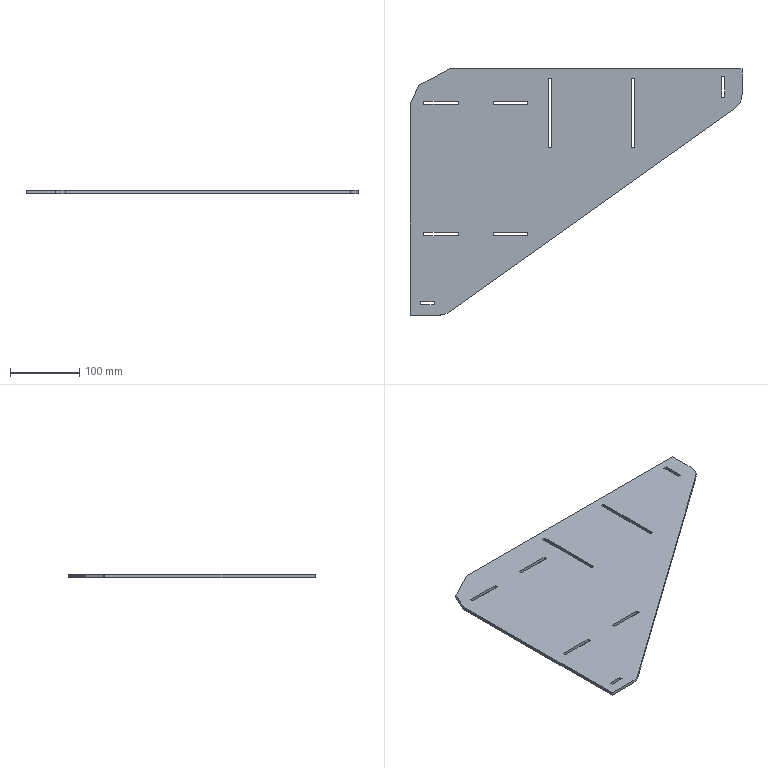Part | SolidWorks | features FlatPattern 1, SMBaseFlange 1, SheetMetal 1 | 1 solid | 44 faces | box 479.97 x 356 x 4.5 mm | volume 459091 mm3 | plane 42 | cylinder 2 | commonest cylinder face diameters 50 x2
STEP:
#1=CARTESIAN_POINT('',(28.5,449.2,0.));
#2=VERTEX_POINT('',#1);
#3=CARTESIAN_POINT('',(70.512,449.2,0.));
#4=VERTEX_POINT('',#3);
#5=CARTESIAN_POINT('',(28.5,449.2,0.));
#6=DIRECTION('',(1.,0.,0.));
#7=VECTOR('',#6,1000.);
#8=LINE('',#5,#7);
#9=EDGE_CURVE('',#2,#4,#8,.T.);
#10=ORIENTED_EDGE('',*,*,#9,.F.);
#11=CARTESIAN_POINT('',(28.5,449.2,-4.5));
#12=VERTEX_POINT('',#11);
#13=CARTESIAN_POINT('',(28.5,449.2,-4.5));
#14=DIRECTION('',(0.,0.,1.));
#15=VECTOR('',#14,1000.);
#16=LINE('',#13,#15);
#17=EDGE_CURVE('',#12,#2,#16,.T.);
#18=ORIENTED_EDGE('',*,*,#17,.F.);
#19=CARTESIAN_POINT('',(70.512,449.2,-4.5));
#20=VERTEX_POINT('',#19);
#21=CARTESIAN_POINT('',(28.5,449.2,-4.5));
#22=DIRECTION('',(1.,0.,0.));
#23=VECTOR('',#22,1000.);
#24=LINE('',#21,#23);
#25=EDGE_CURVE('',#12,#20,#24,.T.);
#26=ORIENTED_EDGE('',*,*,#25,.T.);
#27=CARTESIAN_POINT('',(70.512,449.2,-4.5));
#28=DIRECTION('',(0.,0.,1.));
#29=VECTOR('',#28,1000.);
#30=LINE('',#27,#29);
#31=EDGE_CURVE('',#20,#4,#30,.T.);
#32=ORIENTED_EDGE('',*,*,#31,.T.);
#33=EDGE_LOOP('',(#10,#18,#26,#32));
#34=FACE_OUTER_BOUND('',#33,.T.);
#35=CARTESIAN_POINT('',(28.5,449.2,-4.5));
#36=DIRECTION('',(0.,-1.,0.));
#37=DIRECTION('',(0.,0.,-1.));
#38=AXIS2_PLACEMENT_3D('',#35,#36,#37);
#39=PLANE('',#38);
#40=ADVANCED_FACE('',(#34),#39,.T.);
#41=CARTESIAN_POINT('',(28.5,753.2,0.));
#42=VERTEX_POINT('',#41);
#43=CARTESIAN_POINT('',(28.5,449.2,0.));
#44=DIRECTION('',(0.,-1.,0.));
#45=VECTOR('',#44,1000.);
#46=LINE('',#43,#45);
#47=EDGE_CURVE('',#42,#2,#46,.T.);
#48=ORIENTED_EDGE('',*,*,#47,.F.);
#49=CARTESIAN_POINT('',(28.5,753.2,-4.5));
#50=VERTEX_POINT('',#49);
#51=CARTESIAN_POINT('',(28.5,753.2,-4.5));
#52=DIRECTION('',(0.,0.,1.));
#53=VECTOR('',#52,1000.);
#54=LINE('',#51,#53);
#55=EDGE_CURVE('',#50,#42,#54,.T.);
#56=ORIENTED_EDGE('',*,*,#55,.F.);
#57=CARTESIAN_POINT('',(28.5,449.2,-4.5));
#58=DIRECTION('',(0.,-1.,0.));
#59=VECTOR('',#58,1000.);
#60=LINE('',#57,#59);
#61=EDGE_CURVE('',#50,#12,#60,.T.);
#62=ORIENTED_EDGE('',*,*,#61,.T.);
#63=ORIENTED_EDGE('',*,*,#17,.T.);
#64=EDGE_LOOP('',(#48,#56,#62,#63));
#65=FACE_OUTER_BOUND('',#64,.T.);
#66=CARTESIAN_POINT('',(28.5,449.2,-4.5));
#67=DIRECTION('',(-1.,0.,0.));
#68=DIRECTION('',(0.,0.,1.));
#69=AXIS2_PLACEMENT_3D('',#66,#67,#68);
#70=PLANE('',#69);
#71=ADVANCED_FACE('',(#65),#70,.T.);
#72=CARTESIAN_POINT('',(28.923,755.106,0.));
#73=VERTEX_POINT('',#72);
#74=CARTESIAN_POINT('',(28.5,753.2,0.));
#75=DIRECTION('',(-0.2164,-0.9763,0.));
#76=VECTOR('',#75,1000.);
#77=LINE('',#74,#76);
#78=EDGE_CURVE('',#73,#42,#77,.T.);
#79=ORIENTED_EDGE('',*,*,#78,.F.);
#80=CARTESIAN_POINT('',(28.923,755.106,-4.5));
#81=VERTEX_POINT('',#80);
#82=CARTESIAN_POINT('',(28.923,755.106,-4.5));
#83=DIRECTION('',(0.,0.,1.));
#84=VECTOR('',#83,1000.);
#85=LINE('',#82,#84);
#86=EDGE_CURVE('',#81,#73,#85,.T.);
#87=ORIENTED_EDGE('',*,*,#86,.F.);
#88=CARTESIAN_POINT('',(28.5,753.2,-4.5));
#89=DIRECTION('',(-0.2164,-0.9763,0.));
#90=VECTOR('',#89,1000.);
#91=LINE('',#88,#90);
#92=EDGE_CURVE('',#81,#50,#91,.T.);
#93=ORIENTED_EDGE('',*,*,#92,.T.);
#94=ORIENTED_EDGE('',*,*,#55,.T.);
#95=EDGE_LOOP('',(#79,#87,#93,#94));
#96=FACE_OUTER_BOUND('',#95,.T.);
#97=CARTESIAN_POINT('',(28.5,753.2,-4.5));
#98=DIRECTION('',(-0.9763,0.2164,0.));
#99=DIRECTION('',(-0.2164,-0.9763,0.));
#100=AXIS2_PLACEMENT_3D('',#97,#98,#99);
#101=PLANE('',#100);
#102=ADVANCED_FACE('',(#96),#101,.T.);
#103=CARTESIAN_POINT('',(41.179,781.389,0.));
#104=VERTEX_POINT('',#103);
#105=CARTESIAN_POINT('',(28.923,755.106,0.));
#106=DIRECTION('',(-0.4226,-0.9063,0.));
#107=VECTOR('',#106,1000.);
#108=LINE('',#105,#107);
#109=EDGE_CURVE('',#104,#73,#108,.T.);
#110=ORIENTED_EDGE('',*,*,#109,.F.);
#111=CARTESIAN_POINT('',(41.179,781.389,-4.5));
#112=VERTEX_POINT('',#111);
#113=CARTESIAN_POINT('',(41.179,781.389,-4.5));
#114=DIRECTION('',(0.,0.,1.));
#115=VECTOR('',#114,1000.);
#116=LINE('',#113,#115);
#117=EDGE_CURVE('',#112,#104,#116,.T.);
#118=ORIENTED_EDGE('',*,*,#117,.F.);
#119=CARTESIAN_POINT('',(28.923,755.106,-4.5));
#120=DIRECTION('',(-0.4226,-0.9063,0.));
#121=VECTOR('',#120,1000.);
#122=LINE('',#119,#121);
#123=EDGE_CURVE('',#112,#81,#122,.T.);
#124=ORIENTED_EDGE('',*,*,#123,.T.);
#125=ORIENTED_EDGE('',*,*,#86,.T.);
#126=EDGE_LOOP('',(#110,#118,#124,#125));
#127=FACE_OUTER_BOUND('',#126,.T.);
#128=CARTESIAN_POINT('',(28.923,755.106,-4.5));
#129=DIRECTION('',(-0.9063,0.4226,0.));
#130=DIRECTION('',(-0.4226,-0.9063,0.));
#131=AXIS2_PLACEMENT_3D('',#128,#129,#130);
#132=PLANE('',#131);
#133=ADVANCED_FACE('',(#127),#132,.T.);
#134=CARTESIAN_POINT('',(85.96,805.2,0.));
#135=VERTEX_POINT('',#134);
#136=CARTESIAN_POINT('',(41.179,781.389,0.));
#137=DIRECTION('',(-0.8829,-0.4695,0.));
#138=VECTOR('',#137,1000.);
#139=LINE('',#136,#138);
#140=EDGE_CURVE('',#135,#104,#139,.T.);
#141=ORIENTED_EDGE('',*,*,#140,.F.);
#142=CARTESIAN_POINT('',(85.96,805.2,-4.5));
#143=VERTEX_POINT('',#142);
#144=CARTESIAN_POINT('',(85.96,805.2,-4.5));
#145=DIRECTION('',(0.,0.,1.));
#146=VECTOR('',#145,1000.);
#147=LINE('',#144,#146);
#148=EDGE_CURVE('',#143,#135,#147,.T.);
#149=ORIENTED_EDGE('',*,*,#148,.F.);
#150=CARTESIAN_POINT('',(41.179,781.389,-4.5));
#151=DIRECTION('',(-0.8829,-0.4695,0.));
#152=VECTOR('',#151,1000.);
#153=LINE('',#150,#152);
#154=EDGE_CURVE('',#143,#112,#153,.T.);
#155=ORIENTED_EDGE('',*,*,#154,.T.);
#156=ORIENTED_EDGE('',*,*,#117,.T.);
#157=EDGE_LOOP('',(#141,#149,#155,#156));
#158=FACE_OUTER_BOUND('',#157,.T.);
#159=CARTESIAN_POINT('',(41.179,781.389,-4.5));
#160=DIRECTION('',(-0.4695,0.8829,0.));
#161=DIRECTION('',(-0.8829,-0.4695,0.));
#162=AXIS2_PLACEMENT_3D('',#159,#160,#161);
#163=PLANE('',#162);
#164=ADVANCED_FACE('',(#158),#163,.T.);
#165=CARTESIAN_POINT('',(508.47,805.2,0.));
#166=VERTEX_POINT('',#165);
#167=CARTESIAN_POINT('',(508.47,805.2,0.));
#168=DIRECTION('',(-1.,0.,0.));
#169=VECTOR('',#168,1000.);
#170=LINE('',#167,#169);
#171=EDGE_CURVE('',#166,#135,#170,.T.);
#172=ORIENTED_EDGE('',*,*,#171,.F.);
#173=CARTESIAN_POINT('',(508.47,805.2,-4.5));
#174=VERTEX_POINT('',#173);
#175=CARTESIAN_POINT('',(508.47,805.2,-4.5));
#176=DIRECTION('',(0.,0.,1.));
#177=VECTOR('',#176,1000.);
#178=LINE('',#175,#177);
#179=EDGE_CURVE('',#174,#166,#178,.T.);
#180=ORIENTED_EDGE('',*,*,#179,.F.);
#181=CARTESIAN_POINT('',(508.47,805.2,-4.5));
#182=DIRECTION('',(-1.,0.,0.));
#183=VECTOR('',#182,1000.);
#184=LINE('',#181,#183);
#185=EDGE_CURVE('',#174,#143,#184,.T.);
#186=ORIENTED_EDGE('',*,*,#185,.T.);
#187=ORIENTED_EDGE('',*,*,#148,.T.);
#188=EDGE_LOOP('',(#172,#180,#186,#187));
#189=FACE_OUTER_BOUND('',#188,.T.);
#190=CARTESIAN_POINT('',(508.47,805.2,-4.5));
#191=DIRECTION('',(0.,1.,0.));
#192=DIRECTION('',(0.,0.,1.));
#193=AXIS2_PLACEMENT_3D('',#190,#191,#192);
#194=PLANE('',#193);
#195=ADVANCED_FACE('',(#189),#194,.T.);
#196=CARTESIAN_POINT('',(508.47,768.093,0.));
#197=VERTEX_POINT('',#196);
#198=CARTESIAN_POINT('',(508.47,768.093,0.));
#199=DIRECTION('',(0.,1.,0.));
#200=VECTOR('',#199,1000.);
#201=LINE('',#198,#200);
#202=EDGE_CURVE('',#197,#166,#201,.T.);
#203=ORIENTED_EDGE('',*,*,#202,.F.);
#204=CARTESIAN_POINT('',(508.47,768.093,-4.5));
#205=VERTEX_POINT('',#204);
#206=CARTESIAN_POINT('',(508.47,768.093,-4.5));
#207=DIRECTION('',(0.,0.,1.));
#208=VECTOR('',#207,1000.);
#209=LINE('',#206,#208);
#210=EDGE_CURVE('',#205,#197,#209,.T.);
#211=ORIENTED_EDGE('',*,*,#210,.F.);
#212=CARTESIAN_POINT('',(508.47,768.093,-4.5));
#213=DIRECTION('',(0.,1.,0.));
#214=VECTOR('',#213,1000.);
#215=LINE('',#212,#214);
#216=EDGE_CURVE('',#205,#174,#215,.T.);
#217=ORIENTED_EDGE('',*,*,#216,.T.);
#218=ORIENTED_EDGE('',*,*,#179,.T.);
#219=EDGE_LOOP('',(#203,#211,#217,#218));
#220=FACE_OUTER_BOUND('',#219,.T.);
#221=CARTESIAN_POINT('',(508.47,768.093,-4.5));
#222=DIRECTION('',(1.,0.,0.));
#223=DIRECTION('',(0.,0.,-1.));
#224=AXIS2_PLACEMENT_3D('',#221,#222,#223);
#225=PLANE('',#224);
#226=ADVANCED_FACE('',(#220),#225,.T.);
#227=CARTESIAN_POINT('',(497.966,747.724,0.));
#228=VERTEX_POINT('',#227);
#229=CARTESIAN_POINT('',(483.47,768.093,0.));
#230=DIRECTION('',(0.,0.,1.));
#231=DIRECTION('',(1.,0.,0.));
#232=AXIS2_PLACEMENT_3D('',#229,#230,#231);
#233=CIRCLE('',#232,25.);
#234=EDGE_CURVE('',#228,#197,#233,.T.);
#235=ORIENTED_EDGE('',*,*,#234,.F.);
#236=CARTESIAN_POINT('',(497.966,747.724,-4.5));
#237=VERTEX_POINT('',#236);
#238=CARTESIAN_POINT('',(497.966,747.724,-4.5));
#239=DIRECTION('',(0.,0.,1.));
#240=VECTOR('',#239,1000.);
#241=LINE('',#238,#240);
#242=EDGE_CURVE('',#237,#228,#241,.T.);
#243=ORIENTED_EDGE('',*,*,#242,.F.);
#244=CARTESIAN_POINT('',(483.47,768.093,-4.5));
#245=DIRECTION('',(0.,0.,1.));
#246=DIRECTION('',(1.,0.,0.));
#247=AXIS2_PLACEMENT_3D('',#244,#245,#246);
#248=CIRCLE('',#247,25.);
#249=EDGE_CURVE('',#237,#205,#248,.T.);
#250=ORIENTED_EDGE('',*,*,#249,.T.);
#251=ORIENTED_EDGE('',*,*,#210,.T.);
#252=EDGE_LOOP('',(#235,#243,#250,#251));
#253=FACE_OUTER_BOUND('',#252,.T.);
#254=CARTESIAN_POINT('',(483.47,768.093,-4.5));
#255=DIRECTION('',(0.,0.,1.));
#256=DIRECTION('',(1.,0.,0.));
#257=AXIS2_PLACEMENT_3D('',#254,#255,#256);
#258=CYLINDRICAL_SURFACE('',#257,25.);
#259=ADVANCED_FACE('',(#253),#258,.T.);
#260=CARTESIAN_POINT('',(85.008,453.832,0.));
#261=VERTEX_POINT('',#260);
#262=CARTESIAN_POINT('',(497.966,747.724,0.));
#263=DIRECTION('',(0.8147,0.5798,0.));
#264=VECTOR('',#263,1000.);
#265=LINE('',#262,#264);
#266=EDGE_CURVE('',#261,#228,#265,.T.);
#267=ORIENTED_EDGE('',*,*,#266,.F.);
#268=CARTESIAN_POINT('',(85.008,453.832,-4.5));
#269=VERTEX_POINT('',#268);
#270=CARTESIAN_POINT('',(85.008,453.832,-4.5));
#271=DIRECTION('',(0.,0.,1.));
#272=VECTOR('',#271,1000.);
#273=LINE('',#270,#272);
#274=EDGE_CURVE('',#269,#261,#273,.T.);
#275=ORIENTED_EDGE('',*,*,#274,.F.);
#276=CARTESIAN_POINT('',(497.966,747.724,-4.5));
#277=DIRECTION('',(0.8147,0.5798,0.));
#278=VECTOR('',#277,1000.);
#279=LINE('',#276,#278);
#280=EDGE_CURVE('',#269,#237,#279,.T.);
#281=ORIENTED_EDGE('',*,*,#280,.T.);
#282=ORIENTED_EDGE('',*,*,#242,.T.);
#283=EDGE_LOOP('',(#267,#275,#281,#282));
#284=FACE_OUTER_BOUND('',#283,.T.);
#285=CARTESIAN_POINT('',(497.966,747.724,-4.5));
#286=DIRECTION('',(0.5798,-0.8147,0.));
#287=DIRECTION('',(0.8147,0.5798,0.));
#288=AXIS2_PLACEMENT_3D('',#285,#286,#287);
#289=PLANE('',#288);
#290=ADVANCED_FACE('',(#284),#289,.T.);
#291=CARTESIAN_POINT('',(70.512,474.2,0.));
#292=DIRECTION('',(0.,0.,1.));
#293=DIRECTION('',(1.,0.,0.));
#294=AXIS2_PLACEMENT_3D('',#291,#292,#293);
#295=CIRCLE('',#294,25.);
#296=EDGE_CURVE('',#4,#261,#295,.T.);
#297=ORIENTED_EDGE('',*,*,#296,.F.);
#298=ORIENTED_EDGE('',*,*,#31,.F.);
#299=CARTESIAN_POINT('',(70.512,474.2,-4.5));
#300=DIRECTION('',(0.,0.,1.));
#301=DIRECTION('',(1.,0.,0.));
#302=AXIS2_PLACEMENT_3D('',#299,#300,#301);
#303=CIRCLE('',#302,25.);
#304=EDGE_CURVE('',#20,#269,#303,.T.);
#305=ORIENTED_EDGE('',*,*,#304,.T.);
#306=ORIENTED_EDGE('',*,*,#274,.T.);
#307=EDGE_LOOP('',(#297,#298,#305,#306));
#308=FACE_OUTER_BOUND('',#307,.T.);
#309=CARTESIAN_POINT('',(70.512,474.2,-4.5));
#310=DIRECTION('',(0.,0.,1.));
#311=DIRECTION('',(1.,0.,0.));
#312=AXIS2_PLACEMENT_3D('',#309,#310,#311);
#313=CYLINDRICAL_SURFACE('',#312,25.);
#314=ADVANCED_FACE('',(#308),#313,.T.);
#315=CARTESIAN_POINT('',(43.5,464.2,-4.5));
#316=VERTEX_POINT('',#315);
#317=CARTESIAN_POINT('',(63.5,464.2,-4.5));
#318=VERTEX_POINT('',#317);
#319=CARTESIAN_POINT('',(63.5,464.2,-4.5));
#320=DIRECTION('',(1.,0.,0.));
#321=VECTOR('',#320,1000.);
#322=LINE('',#319,#321);
#323=EDGE_CURVE('',#316,#318,#322,.T.);
#324=ORIENTED_EDGE('',*,*,#323,.T.);
#325=CARTESIAN_POINT('',(63.5,468.7,-4.5));
#326=VERTEX_POINT('',#325);
#327=CARTESIAN_POINT('',(63.5,464.2,-4.5));
#328=DIRECTION('',(0.,1.,0.));
#329=VECTOR('',#328,1000.);
#330=LINE('',#327,#329);
#331=EDGE_CURVE('',#318,#326,#330,.T.);
#332=ORIENTED_EDGE('',*,*,#331,.T.);
#333=CARTESIAN_POINT('',(43.5,468.7,-4.5));
#334=VERTEX_POINT('',#333);
#335=CARTESIAN_POINT('',(63.5,468.7,-4.5));
#336=DIRECTION('',(-1.,0.,0.));
#337=VECTOR('',#336,1000.);
#338=LINE('',#335,#337);
#339=EDGE_CURVE('',#326,#334,#338,.T.);
#340=ORIENTED_EDGE('',*,*,#339,.T.);
#341=CARTESIAN_POINT('',(43.5,464.2,-4.5));
#342=DIRECTION('',(0.,-1.,0.));
#343=VECTOR('',#342,1000.);
#344=LINE('',#341,#343);
#345=EDGE_CURVE('',#334,#316,#344,.T.);
#346=ORIENTED_EDGE('',*,*,#345,.T.);
#347=EDGE_LOOP('',(#324,#332,#340,#346));
#348=FACE_BOUND('',#347,.T.);
#349=CARTESIAN_POINT('',(478.97,764.2,-4.5));
#350=VERTEX_POINT('',#349);
#351=CARTESIAN_POINT('',(483.47,764.2,-4.5));
#352=VERTEX_POINT('',#351);
#353=CARTESIAN_POINT('',(483.47,764.2,-4.5));
#354=DIRECTION('',(1.,0.,0.));
#355=VECTOR('',#354,1000.);
#356=LINE('',#353,#355);
#357=EDGE_CURVE('',#350,#352,#356,.T.);
#358=ORIENTED_EDGE('',*,*,#357,.T.);
#359=CARTESIAN_POINT('',(483.47,794.2,-4.5));
#360=VERTEX_POINT('',#359);
#361=CARTESIAN_POINT('',(483.47,794.2,-4.5));
#362=DIRECTION('',(0.,1.,0.));
#363=VECTOR('',#362,1000.);
#364=LINE('',#361,#363);
#365=EDGE_CURVE('',#352,#360,#364,.T.);
#366=ORIENTED_EDGE('',*,*,#365,.T.);
#367=CARTESIAN_POINT('',(478.97,794.2,-4.5));
#368=VERTEX_POINT('',#367);
#369=CARTESIAN_POINT('',(483.47,794.2,-4.5));
#370=DIRECTION('',(-1.,0.,0.));
#371=VECTOR('',#370,1000.);
#372=LINE('',#369,#371);
#373=EDGE_CURVE('',#360,#368,#372,.T.);
#374=ORIENTED_EDGE('',*,*,#373,.T.);
#375=CARTESIAN_POINT('',(478.97,794.2,-4.5));
#376=DIRECTION('',(0.,-1.,0.));
#377=VECTOR('',#376,1000.);
#378=LINE('',#375,#377);
#379=EDGE_CURVE('',#368,#350,#378,.T.);
#380=ORIENTED_EDGE('',*,*,#379,.T.);
#381=EDGE_LOOP('',(#358,#366,#374,#380));
#382=FACE_BOUND('',#381,.T.);
#383=CARTESIAN_POINT('',(353.47,791.7,-4.5));
#384=VERTEX_POINT('',#383);
#385=CARTESIAN_POINT('',(348.97,791.7,-4.5));
#386=VERTEX_POINT('',#385);
#387=CARTESIAN_POINT('',(348.97,791.7,-4.5));
#388=DIRECTION('',(-1.,0.,0.));
#389=VECTOR('',#388,1000.);
#390=LINE('',#387,#389);
#391=EDGE_CURVE('',#384,#386,#390,.T.);
#392=ORIENTED_EDGE('',*,*,#391,.T.);
#393=CARTESIAN_POINT('',(348.97,691.7,-4.5));
#394=VERTEX_POINT('',#393);
#395=CARTESIAN_POINT('',(348.97,791.7,-4.5));
#396=DIRECTION('',(0.,-1.,0.));
#397=VECTOR('',#396,1000.);
#398=LINE('',#395,#397);
#399=EDGE_CURVE('',#386,#394,#398,.T.);
#400=ORIENTED_EDGE('',*,*,#399,.T.);
#401=CARTESIAN_POINT('',(353.47,691.7,-4.5));
#402=VERTEX_POINT('',#401);
#403=CARTESIAN_POINT('',(348.97,691.7,-4.5));
#404=DIRECTION('',(1.,0.,0.));
#405=VECTOR('',#404,1000.);
#406=LINE('',#403,#405);
#407=EDGE_CURVE('',#394,#402,#406,.T.);
#408=ORIENTED_EDGE('',*,*,#407,.T.);
#409=CARTESIAN_POINT('',(353.47,791.7,-4.5));
#410=DIRECTION('',(0.,1.,0.));
#411=VECTOR('',#410,1000.);
#412=LINE('',#409,#411);
#413=EDGE_CURVE('',#402,#384,#412,.T.);
#414=ORIENTED_EDGE('',*,*,#413,.T.);
#415=EDGE_LOOP('',(#392,#400,#408,#414));
#416=FACE_BOUND('',#415,.T.);
#417=CARTESIAN_POINT('',(228.97,691.7,-4.5));
#418=VERTEX_POINT('',#417);
#419=CARTESIAN_POINT('',(233.47,691.7,-4.5));
#420=VERTEX_POINT('',#419);
#421=CARTESIAN_POINT('',(233.47,691.7,-4.5));
#422=DIRECTION('',(1.,0.,0.));
#423=VECTOR('',#422,1000.);
#424=LINE('',#421,#423);
#425=EDGE_CURVE('',#418,#420,#424,.T.);
#426=ORIENTED_EDGE('',*,*,#425,.T.);
#427=CARTESIAN_POINT('',(233.47,791.7,-4.5));
#428=VERTEX_POINT('',#427);
#429=CARTESIAN_POINT('',(233.47,791.7,-4.5));
#430=DIRECTION('',(0.,1.,0.));
#431=VECTOR('',#430,1000.);
#432=LINE('',#429,#431);
#433=EDGE_CURVE('',#420,#428,#432,.T.);
#434=ORIENTED_EDGE('',*,*,#433,.T.);
#435=CARTESIAN_POINT('',(228.97,791.7,-4.5));
#436=VERTEX_POINT('',#435);
#437=CARTESIAN_POINT('',(233.47,791.7,-4.5));
#438=DIRECTION('',(-1.,0.,0.));
#439=VECTOR('',#438,1000.);
#440=LINE('',#437,#439);
#441=EDGE_CURVE('',#428,#436,#440,.T.);
#442=ORIENTED_EDGE('',*,*,#441,.T.);
#443=CARTESIAN_POINT('',(228.97,791.7,-4.5));
#444=DIRECTION('',(0.,-1.,0.));
#445=VECTOR('',#444,1000.);
#446=LINE('',#443,#445);
#447=EDGE_CURVE('',#436,#418,#446,.T.);
#448=ORIENTED_EDGE('',*,*,#447,.T.);
#449=EDGE_LOOP('',(#426,#434,#442,#448));
#450=FACE_BOUND('',#449,.T.);
#451=CARTESIAN_POINT('',(48.5,564.2,-4.5));
#452=VERTEX_POINT('',#451);
#453=CARTESIAN_POINT('',(98.5,564.2,-4.5));
#454=VERTEX_POINT('',#453);
#455=CARTESIAN_POINT('',(98.5,564.2,-4.5));
#456=DIRECTION('',(1.,0.,0.));
#457=VECTOR('',#456,1000.);
#458=LINE('',#455,#457);
#459=EDGE_CURVE('',#452,#454,#458,.T.);
#460=ORIENTED_EDGE('',*,*,#459,.T.);
#461=CARTESIAN_POINT('',(98.5,568.7,-4.5));
#462=VERTEX_POINT('',#461);
#463=CARTESIAN_POINT('',(98.5,564.2,-4.5));
#464=DIRECTION('',(0.,1.,0.));
#465=VECTOR('',#464,1000.);
#466=LINE('',#463,#465);
#467=EDGE_CURVE('',#454,#462,#466,.T.);
#468=ORIENTED_EDGE('',*,*,#467,.T.);
#469=CARTESIAN_POINT('',(48.5,568.7,-4.5));
#470=VERTEX_POINT('',#469);
#471=CARTESIAN_POINT('',(98.5,568.7,-4.5));
#472=DIRECTION('',(-1.,0.,0.));
#473=VECTOR('',#472,1000.);
#474=LINE('',#471,#473);
#475=EDGE_CURVE('',#462,#470,#474,.T.);
#476=ORIENTED_EDGE('',*,*,#475,.T.);
#477=CARTESIAN_POINT('',(48.5,564.2,-4.5));
#478=DIRECTION('',(0.,-1.,0.));
#479=VECTOR('',#478,1000.);
#480=LINE('',#477,#479);
#481=EDGE_CURVE('',#470,#452,#480,.T.);
#482=ORIENTED_EDGE('',*,*,#481,.T.);
#483=EDGE_LOOP('',(#460,#468,#476,#482));
#484=FACE_BOUND('',#483,.T.);
#485=CARTESIAN_POINT('',(198.5,568.7,-4.5));
#486=VERTEX_POINT('',#485);
#487=CARTESIAN_POINT('',(148.5,568.7,-4.5));
#488=VERTEX_POINT('',#487);
#489=CARTESIAN_POINT('',(148.5,568.7,-4.5));
#490=DIRECTION('',(-1.,0.,0.));
#491=VECTOR('',#490,1000.);
#492=LINE('',#489,#491);
#493=EDGE_CURVE('',#486,#488,#492,.T.);
#494=ORIENTED_EDGE('',*,*,#493,.T.);
#495=CARTESIAN_POINT('',(148.5,564.2,-4.5));
#496=VERTEX_POINT('',#495);
#497=CARTESIAN_POINT('',(148.5,564.2,-4.5));
#498=DIRECTION('',(0.,-1.,0.));
#499=VECTOR('',#498,1000.);
#500=LINE('',#497,#499);
#501=EDGE_CURVE('',#488,#496,#500,.T.);
#502=ORIENTED_EDGE('',*,*,#501,.T.);
#503=CARTESIAN_POINT('',(198.5,564.2,-4.5));
#504=VERTEX_POINT('',#503);
#505=CARTESIAN_POINT('',(148.5,564.2,-4.5));
#506=DIRECTION('',(1.,0.,0.));
#507=VECTOR('',#506,1000.);
#508=LINE('',#505,#507);
#509=EDGE_CURVE('',#496,#504,#508,.T.);
#510=ORIENTED_EDGE('',*,*,#509,.T.);
#511=CARTESIAN_POINT('',(198.5,564.2,-4.5));
#512=DIRECTION('',(0.,1.,0.));
#513=VECTOR('',#512,1000.);
#514=LINE('',#511,#513);
#515=EDGE_CURVE('',#504,#486,#514,.T.);
#516=ORIENTED_EDGE('',*,*,#515,.T.);
#517=EDGE_LOOP('',(#494,#502,#510,#516));
#518=FACE_BOUND('',#517,.T.);
#519=CARTESIAN_POINT('',(198.5,758.7,-4.5));
#520=VERTEX_POINT('',#519);
#521=CARTESIAN_POINT('',(148.5,758.7,-4.5));
#522=VERTEX_POINT('',#521);
#523=CARTESIAN_POINT('',(148.5,758.7,-4.5));
#524=DIRECTION('',(-1.,0.,0.));
#525=VECTOR('',#524,1000.);
#526=LINE('',#523,#525);
#527=EDGE_CURVE('',#520,#522,#526,.T.);
#528=ORIENTED_EDGE('',*,*,#527,.T.);
#529=CARTESIAN_POINT('',(148.5,754.2,-4.5));
#530=VERTEX_POINT('',#529);
#531=CARTESIAN_POINT('',(148.5,754.2,-4.5));
#532=DIRECTION('',(0.,-1.,0.));
#533=VECTOR('',#532,1000.);
#534=LINE('',#531,#533);
#535=EDGE_CURVE('',#522,#530,#534,.T.);
#536=ORIENTED_EDGE('',*,*,#535,.T.);
#537=CARTESIAN_POINT('',(198.5,754.2,-4.5));
#538=VERTEX_POINT('',#537);
#539=CARTESIAN_POINT('',(148.5,754.2,-4.5));
#540=DIRECTION('',(1.,0.,0.));
#541=VECTOR('',#540,1000.);
#542=LINE('',#539,#541);
#543=EDGE_CURVE('',#530,#538,#542,.T.);
#544=ORIENTED_EDGE('',*,*,#543,.T.);
#545=CARTESIAN_POINT('',(198.5,754.2,-4.5));
#546=DIRECTION('',(0.,1.,0.));
#547=VECTOR('',#546,1000.);
#548=LINE('',#545,#547);
#549=EDGE_CURVE('',#538,#520,#548,.T.);
#550=ORIENTED_EDGE('',*,*,#549,.T.);
#551=EDGE_LOOP('',(#528,#536,#544,#550));
#552=FACE_BOUND('',#551,.T.);
#553=CARTESIAN_POINT('',(48.5,754.2,-4.5));
#554=VERTEX_POINT('',#553);
#555=CARTESIAN_POINT('',(98.5,754.2,-4.5));
#556=VERTEX_POINT('',#555);
#557=CARTESIAN_POINT('',(98.5,754.2,-4.5));
#558=DIRECTION('',(1.,0.,0.));
#559=VECTOR('',#558,1000.);
#560=LINE('',#557,#559);
#561=EDGE_CURVE('',#554,#556,#560,.T.);
#562=ORIENTED_EDGE('',*,*,#561,.T.);
#563=CARTESIAN_POINT('',(98.5,758.7,-4.5));
#564=VERTEX_POINT('',#563);
#565=CARTESIAN_POINT('',(98.5,754.2,-4.5));
#566=DIRECTION('',(0.,1.,0.));
#567=VECTOR('',#566,1000.);
#568=LINE('',#565,#567);
#569=EDGE_CURVE('',#556,#564,#568,.T.);
#570=ORIENTED_EDGE('',*,*,#569,.T.);
#571=CARTESIAN_POINT('',(48.5,758.7,-4.5));
#572=VERTEX_POINT('',#571);
#573=CARTESIAN_POINT('',(98.5,758.7,-4.5));
#574=DIRECTION('',(-1.,0.,0.));
#575=VECTOR('',#574,1000.);
#576=LINE('',#573,#575);
#577=EDGE_CURVE('',#564,#572,#576,.T.);
#578=ORIENTED_EDGE('',*,*,#577,.T.);
#579=CARTESIAN_POINT('',(48.5,754.2,-4.5));
#580=DIRECTION('',(0.,-1.,0.));
#581=VECTOR('',#580,1000.);
#582=LINE('',#579,#581);
#583=EDGE_CURVE('',#572,#554,#582,.T.);
#584=ORIENTED_EDGE('',*,*,#583,.T.);
#585=EDGE_LOOP('',(#562,#570,#578,#584));
#586=FACE_BOUND('',#585,.T.);
#587=ORIENTED_EDGE('',*,*,#25,.F.);
#588=ORIENTED_EDGE('',*,*,#61,.F.);
#589=ORIENTED_EDGE('',*,*,#92,.F.);
#590=ORIENTED_EDGE('',*,*,#123,.F.);
#591=ORIENTED_EDGE('',*,*,#154,.F.);
#592=ORIENTED_EDGE('',*,*,#185,.F.);
#593=ORIENTED_EDGE('',*,*,#216,.F.);
#594=ORIENTED_EDGE('',*,*,#249,.F.);
#595=ORIENTED_EDGE('',*,*,#280,.F.);
#596=ORIENTED_EDGE('',*,*,#304,.F.);
#597=EDGE_LOOP('',(#587,#588,#589,#590,#591,#592,#593,#594,#595,#596));
#598=FACE_OUTER_BOUND('',#597,.T.);
#599=CARTESIAN_POINT('',(70.512,474.2,-4.5));
#600=DIRECTION('',(0.,0.,1.));
#601=DIRECTION('',(1.,0.,0.));
#602=AXIS2_PLACEMENT_3D('',#599,#600,#601);
#603=PLANE('',#602);
#604=ADVANCED_FACE('',(#348,#382,#416,#450,#484,#518,#552,#586,#598),#603,.F.);
#605=CARTESIAN_POINT('',(63.5,464.2,0.));
#606=VERTEX_POINT('',#605);
#607=CARTESIAN_POINT('',(63.5,468.7,0.));
#608=VERTEX_POINT('',#607);
#609=CARTESIAN_POINT('',(63.5,464.2,0.));
#610=DIRECTION('',(0.,1.,0.));
#611=VECTOR('',#610,1000.);
#612=LINE('',#609,#611);
#613=EDGE_CURVE('',#606,#608,#612,.T.);
#614=ORIENTED_EDGE('',*,*,#613,.F.);
#615=CARTESIAN_POINT('',(43.5,464.2,0.));
#616=VERTEX_POINT('',#615);
#617=CARTESIAN_POINT('',(63.5,464.2,0.));
#618=DIRECTION('',(1.,0.,0.));
#619=VECTOR('',#618,1000.);
#620=LINE('',#617,#619);
#621=EDGE_CURVE('',#616,#606,#620,.T.);
#622=ORIENTED_EDGE('',*,*,#621,.F.);
#623=CARTESIAN_POINT('',(43.5,468.7,0.));
#624=VERTEX_POINT('',#623);
#625=CARTESIAN_POINT('',(43.5,464.2,0.));
#626=DIRECTION('',(0.,-1.,0.));
#627=VECTOR('',#626,1000.);
#628=LINE('',#625,#627);
#629=EDGE_CURVE('',#624,#616,#628,.T.);
#630=ORIENTED_EDGE('',*,*,#629,.F.);
#631=CARTESIAN_POINT('',(63.5,468.7,0.));
#632=DIRECTION('',(-1.,0.,0.));
#633=VECTOR('',#632,1000.);
#634=LINE('',#631,#633);
#635=EDGE_CURVE('',#608,#624,#634,.T.);
#636=ORIENTED_EDGE('',*,*,#635,.F.);
#637=EDGE_LOOP('',(#614,#622,#630,#636));
#638=FACE_BOUND('',#637,.T.);
#639=CARTESIAN_POINT('',(483.47,764.2,0.));
#640=VERTEX_POINT('',#639);
#641=CARTESIAN_POINT('',(483.47,794.2,0.));
#642=VERTEX_POINT('',#641);
#643=CARTESIAN_POINT('',(483.47,794.2,0.));
#644=DIRECTION('',(0.,1.,0.));
#645=VECTOR('',#644,1000.);
#646=LINE('',#643,#645);
#647=EDGE_CURVE('',#640,#642,#646,.T.);
#648=ORIENTED_EDGE('',*,*,#647,.F.);
#649=CARTESIAN_POINT('',(478.97,764.2,0.));
#650=VERTEX_POINT('',#649);
#651=CARTESIAN_POINT('',(483.47,764.2,0.));
#652=DIRECTION('',(1.,0.,0.));
#653=VECTOR('',#652,1000.);
#654=LINE('',#651,#653);
#655=EDGE_CURVE('',#650,#640,#654,.T.);
#656=ORIENTED_EDGE('',*,*,#655,.F.);
#657=CARTESIAN_POINT('',(478.97,794.2,0.));
#658=VERTEX_POINT('',#657);
#659=CARTESIAN_POINT('',(478.97,794.2,0.));
#660=DIRECTION('',(0.,-1.,0.));
#661=VECTOR('',#660,1000.);
#662=LINE('',#659,#661);
#663=EDGE_CURVE('',#658,#650,#662,.T.);
#664=ORIENTED_EDGE('',*,*,#663,.F.);
#665=CARTESIAN_POINT('',(483.47,794.2,0.));
#666=DIRECTION('',(-1.,0.,0.));
#667=VECTOR('',#666,1000.);
#668=LINE('',#665,#667);
#669=EDGE_CURVE('',#642,#658,#668,.T.);
#670=ORIENTED_EDGE('',*,*,#669,.F.);
#671=EDGE_LOOP('',(#648,#656,#664,#670));
#672=FACE_BOUND('',#671,.T.);
#673=CARTESIAN_POINT('',(348.97,791.7,0.));
#674=VERTEX_POINT('',#673);
#675=CARTESIAN_POINT('',(348.97,691.7,0.));
#676=VERTEX_POINT('',#675);
#677=CARTESIAN_POINT('',(348.97,791.7,0.));
#678=DIRECTION('',(0.,-1.,0.));
#679=VECTOR('',#678,1000.);
#680=LINE('',#677,#679);
#681=EDGE_CURVE('',#674,#676,#680,.T.);
#682=ORIENTED_EDGE('',*,*,#681,.F.);
#683=CARTESIAN_POINT('',(353.47,791.7,0.));
#684=VERTEX_POINT('',#683);
#685=CARTESIAN_POINT('',(348.97,791.7,0.));
#686=DIRECTION('',(-1.,0.,0.));
#687=VECTOR('',#686,1000.);
#688=LINE('',#685,#687);
#689=EDGE_CURVE('',#684,#674,#688,.T.);
#690=ORIENTED_EDGE('',*,*,#689,.F.);
#691=CARTESIAN_POINT('',(353.47,691.7,0.));
#692=VERTEX_POINT('',#691);
#693=CARTESIAN_POINT('',(353.47,791.7,0.));
#694=DIRECTION('',(0.,1.,0.));
#695=VECTOR('',#694,1000.);
#696=LINE('',#693,#695);
#697=EDGE_CURVE('',#692,#684,#696,.T.);
#698=ORIENTED_EDGE('',*,*,#697,.F.);
#699=CARTESIAN_POINT('',(348.97,691.7,0.));
#700=DIRECTION('',(1.,0.,0.));
#701=VECTOR('',#700,1000.);
#702=LINE('',#699,#701);
#703=EDGE_CURVE('',#676,#692,#702,.T.);
#704=ORIENTED_EDGE('',*,*,#703,.F.);
#705=EDGE_LOOP('',(#682,#690,#698,#704));
#706=FACE_BOUND('',#705,.T.);
#707=CARTESIAN_POINT('',(233.47,691.7,0.));
#708=VERTEX_POINT('',#707);
#709=CARTESIAN_POINT('',(233.47,791.7,0.));
#710=VERTEX_POINT('',#709);
#711=CARTESIAN_POINT('',(233.47,791.7,0.));
#712=DIRECTION('',(0.,1.,0.));
#713=VECTOR('',#712,1000.);
#714=LINE('',#711,#713);
#715=EDGE_CURVE('',#708,#710,#714,.T.);
#716=ORIENTED_EDGE('',*,*,#715,.F.);
#717=CARTESIAN_POINT('',(228.97,691.7,0.));
#718=VERTEX_POINT('',#717);
#719=CARTESIAN_POINT('',(233.47,691.7,0.));
#720=DIRECTION('',(1.,0.,0.));
#721=VECTOR('',#720,1000.);
#722=LINE('',#719,#721);
#723=EDGE_CURVE('',#718,#708,#722,.T.);
#724=ORIENTED_EDGE('',*,*,#723,.F.);
#725=CARTESIAN_POINT('',(228.97,791.7,0.));
#726=VERTEX_POINT('',#725);
#727=CARTESIAN_POINT('',(228.97,791.7,0.));
#728=DIRECTION('',(0.,-1.,0.));
#729=VECTOR('',#728,1000.);
#730=LINE('',#727,#729);
#731=EDGE_CURVE('',#726,#718,#730,.T.);
#732=ORIENTED_EDGE('',*,*,#731,.F.);
#733=CARTESIAN_POINT('',(233.47,791.7,0.));
#734=DIRECTION('',(-1.,0.,0.));
#735=VECTOR('',#734,1000.);
#736=LINE('',#733,#735);
#737=EDGE_CURVE('',#710,#726,#736,.T.);
#738=ORIENTED_EDGE('',*,*,#737,.F.);
#739=EDGE_LOOP('',(#716,#724,#732,#738));
#740=FACE_BOUND('',#739,.T.);
#741=CARTESIAN_POINT('',(98.5,564.2,0.));
#742=VERTEX_POINT('',#741);
#743=CARTESIAN_POINT('',(98.5,568.7,0.));
#744=VERTEX_POINT('',#743);
#745=CARTESIAN_POINT('',(98.5,564.2,0.));
#746=DIRECTION('',(0.,1.,0.));
#747=VECTOR('',#746,1000.);
#748=LINE('',#745,#747);
#749=EDGE_CURVE('',#742,#744,#748,.T.);
#750=ORIENTED_EDGE('',*,*,#749,.F.);
#751=CARTESIAN_POINT('',(48.5,564.2,0.));
#752=VERTEX_POINT('',#751);
#753=CARTESIAN_POINT('',(98.5,564.2,0.));
#754=DIRECTION('',(1.,0.,0.));
#755=VECTOR('',#754,1000.);
#756=LINE('',#753,#755);
#757=EDGE_CURVE('',#752,#742,#756,.T.);
#758=ORIENTED_EDGE('',*,*,#757,.F.);
#759=CARTESIAN_POINT('',(48.5,568.7,0.));
#760=VERTEX_POINT('',#759);
#761=CARTESIAN_POINT('',(48.5,564.2,0.));
#762=DIRECTION('',(0.,-1.,0.));
#763=VECTOR('',#762,1000.);
#764=LINE('',#761,#763);
#765=EDGE_CURVE('',#760,#752,#764,.T.);
#766=ORIENTED_EDGE('',*,*,#765,.F.);
#767=CARTESIAN_POINT('',(98.5,568.7,0.));
#768=DIRECTION('',(-1.,0.,0.));
#769=VECTOR('',#768,1000.);
#770=LINE('',#767,#769);
#771=EDGE_CURVE('',#744,#760,#770,.T.);
#772=ORIENTED_EDGE('',*,*,#771,.F.);
#773=EDGE_LOOP('',(#750,#758,#766,#772));
#774=FACE_BOUND('',#773,.T.);
#775=CARTESIAN_POINT('',(148.5,568.7,0.));
#776=VERTEX_POINT('',#775);
#777=CARTESIAN_POINT('',(148.5,564.2,0.));
#778=VERTEX_POINT('',#777);
#779=CARTESIAN_POINT('',(148.5,564.2,0.));
#780=DIRECTION('',(0.,-1.,0.));
#781=VECTOR('',#780,1000.);
#782=LINE('',#779,#781);
#783=EDGE_CURVE('',#776,#778,#782,.T.);
#784=ORIENTED_EDGE('',*,*,#783,.F.);
#785=CARTESIAN_POINT('',(198.5,568.7,0.));
#786=VERTEX_POINT('',#785);
#787=CARTESIAN_POINT('',(148.5,568.7,0.));
#788=DIRECTION('',(-1.,0.,0.));
#789=VECTOR('',#788,1000.);
#790=LINE('',#787,#789);
#791=EDGE_CURVE('',#786,#776,#790,.T.);
#792=ORIENTED_EDGE('',*,*,#791,.F.);
#793=CARTESIAN_POINT('',(198.5,564.2,0.));
#794=VERTEX_POINT('',#793);
#795=CARTESIAN_POINT('',(198.5,564.2,0.));
#796=DIRECTION('',(0.,1.,0.));
#797=VECTOR('',#796,1000.);
#798=LINE('',#795,#797);
#799=EDGE_CURVE('',#794,#786,#798,.T.);
#800=ORIENTED_EDGE('',*,*,#799,.F.);
#801=CARTESIAN_POINT('',(148.5,564.2,0.));
#802=DIRECTION('',(1.,0.,0.));
#803=VECTOR('',#802,1000.);
#804=LINE('',#801,#803);
#805=EDGE_CURVE('',#778,#794,#804,.T.);
#806=ORIENTED_EDGE('',*,*,#805,.F.);
#807=EDGE_LOOP('',(#784,#792,#800,#806));
#808=FACE_BOUND('',#807,.T.);
#809=CARTESIAN_POINT('',(148.5,758.7,0.));
#810=VERTEX_POINT('',#809);
#811=CARTESIAN_POINT('',(148.5,754.2,0.));
#812=VERTEX_POINT('',#811);
#813=CARTESIAN_POINT('',(148.5,754.2,0.));
#814=DIRECTION('',(0.,-1.,0.));
#815=VECTOR('',#814,1000.);
#816=LINE('',#813,#815);
#817=EDGE_CURVE('',#810,#812,#816,.T.);
#818=ORIENTED_EDGE('',*,*,#817,.F.);
#819=CARTESIAN_POINT('',(198.5,758.7,0.));
#820=VERTEX_POINT('',#819);
#821=CARTESIAN_POINT('',(148.5,758.7,0.));
#822=DIRECTION('',(-1.,0.,0.));
#823=VECTOR('',#822,1000.);
#824=LINE('',#821,#823);
#825=EDGE_CURVE('',#820,#810,#824,.T.);
#826=ORIENTED_EDGE('',*,*,#825,.F.);
#827=CARTESIAN_POINT('',(198.5,754.2,0.));
#828=VERTEX_POINT('',#827);
#829=CARTESIAN_POINT('',(198.5,754.2,0.));
#830=DIRECTION('',(0.,1.,0.));
#831=VECTOR('',#830,1000.);
#832=LINE('',#829,#831);
#833=EDGE_CURVE('',#828,#820,#832,.T.);
#834=ORIENTED_EDGE('',*,*,#833,.F.);
#835=CARTESIAN_POINT('',(148.5,754.2,0.));
#836=DIRECTION('',(1.,0.,0.));
#837=VECTOR('',#836,1000.);
#838=LINE('',#835,#837);
#839=EDGE_CURVE('',#812,#828,#838,.T.);
#840=ORIENTED_EDGE('',*,*,#839,.F.);
#841=EDGE_LOOP('',(#818,#826,#834,#840));
#842=FACE_BOUND('',#841,.T.);
#843=CARTESIAN_POINT('',(98.5,754.2,0.));
#844=VERTEX_POINT('',#843);
#845=CARTESIAN_POINT('',(98.5,758.7,0.));
#846=VERTEX_POINT('',#845);
#847=CARTESIAN_POINT('',(98.5,754.2,0.));
#848=DIRECTION('',(0.,1.,0.));
#849=VECTOR('',#848,1000.);
#850=LINE('',#847,#849);
#851=EDGE_CURVE('',#844,#846,#850,.T.);
#852=ORIENTED_EDGE('',*,*,#851,.F.);
#853=CARTESIAN_POINT('',(48.5,754.2,0.));
#854=VERTEX_POINT('',#853);
#855=CARTESIAN_POINT('',(98.5,754.2,0.));
#856=DIRECTION('',(1.,0.,0.));
#857=VECTOR('',#856,1000.);
#858=LINE('',#855,#857);
#859=EDGE_CURVE('',#854,#844,#858,.T.);
#860=ORIENTED_EDGE('',*,*,#859,.F.);
#861=CARTESIAN_POINT('',(48.5,758.7,0.));
#862=VERTEX_POINT('',#861);
#863=CARTESIAN_POINT('',(48.5,754.2,0.));
#864=DIRECTION('',(0.,-1.,0.));
#865=VECTOR('',#864,1000.);
#866=LINE('',#863,#865);
#867=EDGE_CURVE('',#862,#854,#866,.T.);
#868=ORIENTED_EDGE('',*,*,#867,.F.);
#869=CARTESIAN_POINT('',(98.5,758.7,0.));
#870=DIRECTION('',(-1.,0.,0.));
#871=VECTOR('',#870,1000.);
#872=LINE('',#869,#871);
#873=EDGE_CURVE('',#846,#862,#872,.T.);
#874=ORIENTED_EDGE('',*,*,#873,.F.);
#875=EDGE_LOOP('',(#852,#860,#868,#874));
#876=FACE_BOUND('',#875,.T.);
#877=ORIENTED_EDGE('',*,*,#9,.T.);
#878=ORIENTED_EDGE('',*,*,#296,.T.);
#879=ORIENTED_EDGE('',*,*,#266,.T.);
#880=ORIENTED_EDGE('',*,*,#234,.T.);
#881=ORIENTED_EDGE('',*,*,#202,.T.);
#882=ORIENTED_EDGE('',*,*,#171,.T.);
#883=ORIENTED_EDGE('',*,*,#140,.T.);
#884=ORIENTED_EDGE('',*,*,#109,.T.);
#885=ORIENTED_EDGE('',*,*,#78,.T.);
#886=ORIENTED_EDGE('',*,*,#47,.T.);
#887=EDGE_LOOP('',(#877,#878,#879,#880,#881,#882,#883,#884,#885,#886));
#888=FACE_OUTER_BOUND('',#887,.T.);
#889=CARTESIAN_POINT('',(70.512,474.2,0.));
#890=DIRECTION('',(0.,0.,1.));
#891=DIRECTION('',(1.,0.,0.));
#892=AXIS2_PLACEMENT_3D('',#889,#890,#891);
#893=PLANE('',#892);
#894=ADVANCED_FACE('',(#638,#672,#706,#740,#774,#808,#842,#876,#888),#893,.T.);
#895=ORIENTED_EDGE('',*,*,#851,.T.);
#896=CARTESIAN_POINT('',(98.5,758.7,-4.5));
#897=DIRECTION('',(0.,0.,1.));
#898=VECTOR('',#897,1000.);
#899=LINE('',#896,#898);
#900=EDGE_CURVE('',#564,#846,#899,.T.);
#901=ORIENTED_EDGE('',*,*,#900,.F.);
#902=ORIENTED_EDGE('',*,*,#569,.F.);
#903=CARTESIAN_POINT('',(98.5,754.2,-4.5));
#904=DIRECTION('',(0.,0.,1.));
#905=VECTOR('',#904,1000.);
#906=LINE('',#903,#905);
#907=EDGE_CURVE('',#556,#844,#906,.T.);
#908=ORIENTED_EDGE('',*,*,#907,.T.);
#909=EDGE_LOOP('',(#895,#901,#902,#908));
#910=FACE_OUTER_BOUND('',#909,.T.);
#911=CARTESIAN_POINT('',(98.5,754.2,-4.5));
#912=DIRECTION('',(1.,0.,0.));
#913=DIRECTION('',(0.,0.,-1.));
#914=AXIS2_PLACEMENT_3D('',#911,#912,#913);
#915=PLANE('',#914);
#916=ADVANCED_FACE('',(#910),#915,.F.);
#917=ORIENTED_EDGE('',*,*,#859,.T.);
#918=ORIENTED_EDGE('',*,*,#907,.F.);
#919=ORIENTED_EDGE('',*,*,#561,.F.);
#920=CARTESIAN_POINT('',(48.5,754.2,-4.5));
#921=DIRECTION('',(0.,0.,1.));
#922=VECTOR('',#921,1000.);
#923=LINE('',#920,#922);
#924=EDGE_CURVE('',#554,#854,#923,.T.);
#925=ORIENTED_EDGE('',*,*,#924,.T.);
#926=EDGE_LOOP('',(#917,#918,#919,#925));
#927=FACE_OUTER_BOUND('',#926,.T.);
#928=CARTESIAN_POINT('',(98.5,754.2,-4.5));
#929=DIRECTION('',(0.,-1.,0.));
#930=DIRECTION('',(0.,0.,-1.));
#931=AXIS2_PLACEMENT_3D('',#928,#929,#930);
#932=PLANE('',#931);
#933=ADVANCED_FACE('',(#927),#932,.F.);
#934=ORIENTED_EDGE('',*,*,#867,.T.);
#935=ORIENTED_EDGE('',*,*,#924,.F.);
#936=ORIENTED_EDGE('',*,*,#583,.F.);
#937=CARTESIAN_POINT('',(48.5,758.7,-4.5));
#938=DIRECTION('',(0.,0.,1.));
#939=VECTOR('',#938,1000.);
#940=LINE('',#937,#939);
#941=EDGE_CURVE('',#572,#862,#940,.T.);
#942=ORIENTED_EDGE('',*,*,#941,.T.);
#943=EDGE_LOOP('',(#934,#935,#936,#942));
#944=FACE_OUTER_BOUND('',#943,.T.);
#945=CARTESIAN_POINT('',(48.5,754.2,-4.5));
#946=DIRECTION('',(-1.,0.,0.));
#947=DIRECTION('',(0.,0.,1.));
#948=AXIS2_PLACEMENT_3D('',#945,#946,#947);
#949=PLANE('',#948);
#950=ADVANCED_FACE('',(#944),#949,.F.);
#951=ORIENTED_EDGE('',*,*,#873,.T.);
#952=ORIENTED_EDGE('',*,*,#941,.F.);
#953=ORIENTED_EDGE('',*,*,#577,.F.);
#954=ORIENTED_EDGE('',*,*,#900,.T.);
#955=EDGE_LOOP('',(#951,#952,#953,#954));
#956=FACE_OUTER_BOUND('',#955,.T.);
#957=CARTESIAN_POINT('',(98.5,758.7,-4.5));
#958=DIRECTION('',(0.,1.,0.));
#959=DIRECTION('',(0.,0.,1.));
#960=AXIS2_PLACEMENT_3D('',#957,#958,#959);
#961=PLANE('',#960);
#962=ADVANCED_FACE('',(#956),#961,.F.);
#963=ORIENTED_EDGE('',*,*,#817,.T.);
#964=CARTESIAN_POINT('',(148.5,754.2,-4.5));
#965=DIRECTION('',(0.,0.,1.));
#966=VECTOR('',#965,1000.);
#967=LINE('',#964,#966);
#968=EDGE_CURVE('',#530,#812,#967,.T.);
#969=ORIENTED_EDGE('',*,*,#968,.F.);
#970=ORIENTED_EDGE('',*,*,#535,.F.);
#971=CARTESIAN_POINT('',(148.5,758.7,-4.5));
#972=DIRECTION('',(0.,0.,1.));
#973=VECTOR('',#972,1000.);
#974=LINE('',#971,#973);
#975=EDGE_CURVE('',#522,#810,#974,.T.);
#976=ORIENTED_EDGE('',*,*,#975,.T.);
#977=EDGE_LOOP('',(#963,#969,#970,#976));
#978=FACE_OUTER_BOUND('',#977,.T.);
#979=CARTESIAN_POINT('',(148.5,754.2,-4.5));
#980=DIRECTION('',(-1.,0.,0.));
#981=DIRECTION('',(0.,0.,1.));
#982=AXIS2_PLACEMENT_3D('',#979,#980,#981);
#983=PLANE('',#982);
#984=ADVANCED_FACE('',(#978),#983,.F.);
#985=ORIENTED_EDGE('',*,*,#825,.T.);
#986=ORIENTED_EDGE('',*,*,#975,.F.);
#987=ORIENTED_EDGE('',*,*,#527,.F.);
#988=CARTESIAN_POINT('',(198.5,758.7,-4.5));
#989=DIRECTION('',(0.,0.,1.));
#990=VECTOR('',#989,1000.);
#991=LINE('',#988,#990);
#992=EDGE_CURVE('',#520,#820,#991,.T.);
#993=ORIENTED_EDGE('',*,*,#992,.T.);
#994=EDGE_LOOP('',(#985,#986,#987,#993));
#995=FACE_OUTER_BOUND('',#994,.T.);
#996=CARTESIAN_POINT('',(148.5,758.7,-4.5));
#997=DIRECTION('',(0.,1.,0.));
#998=DIRECTION('',(0.,0.,1.));
#999=AXIS2_PLACEMENT_3D('',#996,#997,#998);
#1000=PLANE('',#999);
#1001=ADVANCED_FACE('',(#995),#1000,.F.);
#1002=ORIENTED_EDGE('',*,*,#833,.T.);
#1003=ORIENTED_EDGE('',*,*,#992,.F.);
#1004=ORIENTED_EDGE('',*,*,#549,.F.);
#1005=CARTESIAN_POINT('',(198.5,754.2,-4.5));
#1006=DIRECTION('',(0.,0.,1.));
#1007=VECTOR('',#1006,1000.);
#1008=LINE('',#1005,#1007);
#1009=EDGE_CURVE('',#538,#828,#1008,.T.);
#1010=ORIENTED_EDGE('',*,*,#1009,.T.);
#1011=EDGE_LOOP('',(#1002,#1003,#1004,#1010));
#1012=FACE_OUTER_BOUND('',#1011,.T.);
#1013=CARTESIAN_POINT('',(198.5,754.2,-4.5));
#1014=DIRECTION('',(1.,0.,0.));
#1015=DIRECTION('',(0.,0.,-1.));
#1016=AXIS2_PLACEMENT_3D('',#1013,#1014,#1015);
#1017=PLANE('',#1016);
#1018=ADVANCED_FACE('',(#1012),#1017,.F.);
#1019=ORIENTED_EDGE('',*,*,#839,.T.);
#1020=ORIENTED_EDGE('',*,*,#1009,.F.);
#1021=ORIENTED_EDGE('',*,*,#543,.F.);
#1022=ORIENTED_EDGE('',*,*,#968,.T.);
#1023=EDGE_LOOP('',(#1019,#1020,#1021,#1022));
#1024=FACE_OUTER_BOUND('',#1023,.T.);
#1025=CARTESIAN_POINT('',(148.5,754.2,-4.5));
#1026=DIRECTION('',(0.,-1.,0.));
#1027=DIRECTION('',(0.,0.,-1.));
#1028=AXIS2_PLACEMENT_3D('',#1025,#1026,#1027);
#1029=PLANE('',#1028);
#1030=ADVANCED_FACE('',(#1024),#1029,.F.);
#1031=ORIENTED_EDGE('',*,*,#783,.T.);
#1032=CARTESIAN_POINT('',(148.5,564.2,-4.5));
#1033=DIRECTION('',(0.,0.,1.));
#1034=VECTOR('',#1033,1000.);
#1035=LINE('',#1032,#1034);
#1036=EDGE_CURVE('',#496,#778,#1035,.T.);
#1037=ORIENTED_EDGE('',*,*,#1036,.F.);
#1038=ORIENTED_EDGE('',*,*,#501,.F.);
#1039=CARTESIAN_POINT('',(148.5,568.7,-4.5));
#1040=DIRECTION('',(0.,0.,1.));
#1041=VECTOR('',#1040,1000.);
#1042=LINE('',#1039,#1041);
#1043=EDGE_CURVE('',#488,#776,#1042,.T.);
#1044=ORIENTED_EDGE('',*,*,#1043,.T.);
#1045=EDGE_LOOP('',(#1031,#1037,#1038,#1044));
#1046=FACE_OUTER_BOUND('',#1045,.T.);
#1047=CARTESIAN_POINT('',(148.5,564.2,-4.5));
#1048=DIRECTION('',(-1.,0.,0.));
#1049=DIRECTION('',(0.,0.,1.));
#1050=AXIS2_PLACEMENT_3D('',#1047,#1048,#1049);
#1051=PLANE('',#1050);
#1052=ADVANCED_FACE('',(#1046),#1051,.F.);
#1053=ORIENTED_EDGE('',*,*,#791,.T.);
#1054=ORIENTED_EDGE('',*,*,#1043,.F.);
#1055=ORIENTED_EDGE('',*,*,#493,.F.);
#1056=CARTESIAN_POINT('',(198.5,568.7,-4.5));
#1057=DIRECTION('',(0.,0.,1.));
#1058=VECTOR('',#1057,1000.);
#1059=LINE('',#1056,#1058);
#1060=EDGE_CURVE('',#486,#786,#1059,.T.);
#1061=ORIENTED_EDGE('',*,*,#1060,.T.);
#1062=EDGE_LOOP('',(#1053,#1054,#1055,#1061));
#1063=FACE_OUTER_BOUND('',#1062,.T.);
#1064=CARTESIAN_POINT('',(148.5,568.7,-4.5));
#1065=DIRECTION('',(0.,1.,0.));
#1066=DIRECTION('',(0.,0.,1.));
#1067=AXIS2_PLACEMENT_3D('',#1064,#1065,#1066);
#1068=PLANE('',#1067);
#1069=ADVANCED_FACE('',(#1063),#1068,.F.);
#1070=ORIENTED_EDGE('',*,*,#799,.T.);
#1071=ORIENTED_EDGE('',*,*,#1060,.F.);
#1072=ORIENTED_EDGE('',*,*,#515,.F.);
#1073=CARTESIAN_POINT('',(198.5,564.2,-4.5));
#1074=DIRECTION('',(0.,0.,1.));
#1075=VECTOR('',#1074,1000.);
#1076=LINE('',#1073,#1075);
#1077=EDGE_CURVE('',#504,#794,#1076,.T.);
#1078=ORIENTED_EDGE('',*,*,#1077,.T.);
#1079=EDGE_LOOP('',(#1070,#1071,#1072,#1078));
#1080=FACE_OUTER_BOUND('',#1079,.T.);
#1081=CARTESIAN_POINT('',(198.5,564.2,-4.5));
#1082=DIRECTION('',(1.,0.,0.));
#1083=DIRECTION('',(0.,0.,-1.));
#1084=AXIS2_PLACEMENT_3D('',#1081,#1082,#1083);
#1085=PLANE('',#1084);
#1086=ADVANCED_FACE('',(#1080),#1085,.F.);
#1087=ORIENTED_EDGE('',*,*,#805,.T.);
#1088=ORIENTED_EDGE('',*,*,#1077,.F.);
#1089=ORIENTED_EDGE('',*,*,#509,.F.);
#1090=ORIENTED_EDGE('',*,*,#1036,.T.);
#1091=EDGE_LOOP('',(#1087,#1088,#1089,#1090));
#1092=FACE_OUTER_BOUND('',#1091,.T.);
#1093=CARTESIAN_POINT('',(148.5,564.2,-4.5));
#1094=DIRECTION('',(0.,-1.,0.));
#1095=DIRECTION('',(0.,0.,-1.));
#1096=AXIS2_PLACEMENT_3D('',#1093,#1094,#1095);
#1097=PLANE('',#1096);
#1098=ADVANCED_FACE('',(#1092),#1097,.F.);
#1099=ORIENTED_EDGE('',*,*,#749,.T.);
#1100=CARTESIAN_POINT('',(98.5,568.7,-4.5));
#1101=DIRECTION('',(0.,0.,1.));
#1102=VECTOR('',#1101,1000.);
#1103=LINE('',#1100,#1102);
#1104=EDGE_CURVE('',#462,#744,#1103,.T.);
#1105=ORIENTED_EDGE('',*,*,#1104,.F.);
#1106=ORIENTED_EDGE('',*,*,#467,.F.);
#1107=CARTESIAN_POINT('',(98.5,564.2,-4.5));
#1108=DIRECTION('',(0.,0.,1.));
#1109=VECTOR('',#1108,1000.);
#1110=LINE('',#1107,#1109);
#1111=EDGE_CURVE('',#454,#742,#1110,.T.);
#1112=ORIENTED_EDGE('',*,*,#1111,.T.);
#1113=EDGE_LOOP('',(#1099,#1105,#1106,#1112));
#1114=FACE_OUTER_BOUND('',#1113,.T.);
#1115=CARTESIAN_POINT('',(98.5,564.2,-4.5));
#1116=DIRECTION('',(1.,0.,0.));
#1117=DIRECTION('',(0.,0.,-1.));
#1118=AXIS2_PLACEMENT_3D('',#1115,#1116,#1117);
#1119=PLANE('',#1118);
#1120=ADVANCED_FACE('',(#1114),#1119,.F.);
#1121=ORIENTED_EDGE('',*,*,#757,.T.);
#1122=ORIENTED_EDGE('',*,*,#1111,.F.);
#1123=ORIENTED_EDGE('',*,*,#459,.F.);
#1124=CARTESIAN_POINT('',(48.5,564.2,-4.5));
#1125=DIRECTION('',(0.,0.,1.));
#1126=VECTOR('',#1125,1000.);
#1127=LINE('',#1124,#1126);
#1128=EDGE_CURVE('',#452,#752,#1127,.T.);
#1129=ORIENTED_EDGE('',*,*,#1128,.T.);
#1130=EDGE_LOOP('',(#1121,#1122,#1123,#1129));
#1131=FACE_OUTER_BOUND('',#1130,.T.);
#1132=CARTESIAN_POINT('',(98.5,564.2,-4.5));
#1133=DIRECTION('',(0.,-1.,0.));
#1134=DIRECTION('',(0.,0.,-1.));
#1135=AXIS2_PLACEMENT_3D('',#1132,#1133,#1134);
#1136=PLANE('',#1135);
#1137=ADVANCED_FACE('',(#1131),#1136,.F.);
#1138=ORIENTED_EDGE('',*,*,#765,.T.);
#1139=ORIENTED_EDGE('',*,*,#1128,.F.);
#1140=ORIENTED_EDGE('',*,*,#481,.F.);
#1141=CARTESIAN_POINT('',(48.5,568.7,-4.5));
#1142=DIRECTION('',(0.,0.,1.));
#1143=VECTOR('',#1142,1000.);
#1144=LINE('',#1141,#1143);
#1145=EDGE_CURVE('',#470,#760,#1144,.T.);
#1146=ORIENTED_EDGE('',*,*,#1145,.T.);
#1147=EDGE_LOOP('',(#1138,#1139,#1140,#1146));
#1148=FACE_OUTER_BOUND('',#1147,.T.);
#1149=CARTESIAN_POINT('',(48.5,564.2,-4.5));
#1150=DIRECTION('',(-1.,0.,0.));
#1151=DIRECTION('',(0.,0.,1.));
#1152=AXIS2_PLACEMENT_3D('',#1149,#1150,#1151);
#1153=PLANE('',#1152);
#1154=ADVANCED_FACE('',(#1148),#1153,.F.);
#1155=ORIENTED_EDGE('',*,*,#771,.T.);
#1156=ORIENTED_EDGE('',*,*,#1145,.F.);
#1157=ORIENTED_EDGE('',*,*,#475,.F.);
#1158=ORIENTED_EDGE('',*,*,#1104,.T.);
#1159=EDGE_LOOP('',(#1155,#1156,#1157,#1158));
#1160=FACE_OUTER_BOUND('',#1159,.T.);
#1161=CARTESIAN_POINT('',(98.5,568.7,-4.5));
#1162=DIRECTION('',(0.,1.,0.));
#1163=DIRECTION('',(0.,0.,1.));
#1164=AXIS2_PLACEMENT_3D('',#1161,#1162,#1163);
#1165=PLANE('',#1164);
#1166=ADVANCED_FACE('',(#1160),#1165,.F.);
#1167=ORIENTED_EDGE('',*,*,#715,.T.);
#1168=CARTESIAN_POINT('',(233.47,791.7,-4.5));
#1169=DIRECTION('',(0.,0.,1.));
#1170=VECTOR('',#1169,1000.);
#1171=LINE('',#1168,#1170);
#1172=EDGE_CURVE('',#428,#710,#1171,.T.);
#1173=ORIENTED_EDGE('',*,*,#1172,.F.);
#1174=ORIENTED_EDGE('',*,*,#433,.F.);
#1175=CARTESIAN_POINT('',(233.47,691.7,-4.5));
#1176=DIRECTION('',(0.,0.,1.));
#1177=VECTOR('',#1176,1000.);
#1178=LINE('',#1175,#1177);
#1179=EDGE_CURVE('',#420,#708,#1178,.T.);
#1180=ORIENTED_EDGE('',*,*,#1179,.T.);
#1181=EDGE_LOOP('',(#1167,#1173,#1174,#1180));
#1182=FACE_OUTER_BOUND('',#1181,.T.);
#1183=CARTESIAN_POINT('',(233.47,791.7,-4.5));
#1184=DIRECTION('',(1.,0.,0.));
#1185=DIRECTION('',(0.,0.,-1.));
#1186=AXIS2_PLACEMENT_3D('',#1183,#1184,#1185);
#1187=PLANE('',#1186);
#1188=ADVANCED_FACE('',(#1182),#1187,.F.);
#1189=ORIENTED_EDGE('',*,*,#723,.T.);
#1190=ORIENTED_EDGE('',*,*,#1179,.F.);
#1191=ORIENTED_EDGE('',*,*,#425,.F.);
#1192=CARTESIAN_POINT('',(228.97,691.7,-4.5));
#1193=DIRECTION('',(0.,0.,1.));
#1194=VECTOR('',#1193,1000.);
#1195=LINE('',#1192,#1194);
#1196=EDGE_CURVE('',#418,#718,#1195,.T.);
#1197=ORIENTED_EDGE('',*,*,#1196,.T.);
#1198=EDGE_LOOP('',(#1189,#1190,#1191,#1197));
#1199=FACE_OUTER_BOUND('',#1198,.T.);
#1200=CARTESIAN_POINT('',(233.47,691.7,-4.5));
#1201=DIRECTION('',(0.,-1.,0.));
#1202=DIRECTION('',(0.,0.,-1.));
#1203=AXIS2_PLACEMENT_3D('',#1200,#1201,#1202);
#1204=PLANE('',#1203);
#1205=ADVANCED_FACE('',(#1199),#1204,.F.);
#1206=ORIENTED_EDGE('',*,*,#731,.T.);
#1207=ORIENTED_EDGE('',*,*,#1196,.F.);
#1208=ORIENTED_EDGE('',*,*,#447,.F.);
#1209=CARTESIAN_POINT('',(228.97,791.7,-4.5));
#1210=DIRECTION('',(0.,0.,1.));
#1211=VECTOR('',#1210,1000.);
#1212=LINE('',#1209,#1211);
#1213=EDGE_CURVE('',#436,#726,#1212,.T.);
#1214=ORIENTED_EDGE('',*,*,#1213,.T.);
#1215=EDGE_LOOP('',(#1206,#1207,#1208,#1214));
#1216=FACE_OUTER_BOUND('',#1215,.T.);
#1217=CARTESIAN_POINT('',(228.97,791.7,-4.5));
#1218=DIRECTION('',(-1.,0.,0.));
#1219=DIRECTION('',(0.,0.,1.));
#1220=AXIS2_PLACEMENT_3D('',#1217,#1218,#1219);
#1221=PLANE('',#1220);
#1222=ADVANCED_FACE('',(#1216),#1221,.F.);
#1223=ORIENTED_EDGE('',*,*,#737,.T.);
#1224=ORIENTED_EDGE('',*,*,#1213,.F.);
#1225=ORIENTED_EDGE('',*,*,#441,.F.);
#1226=ORIENTED_EDGE('',*,*,#1172,.T.);
#1227=EDGE_LOOP('',(#1223,#1224,#1225,#1226));
#1228=FACE_OUTER_BOUND('',#1227,.T.);
#1229=CARTESIAN_POINT('',(233.47,791.7,-4.5));
#1230=DIRECTION('',(0.,1.,0.));
#1231=DIRECTION('',(0.,0.,1.));
#1232=AXIS2_PLACEMENT_3D('',#1229,#1230,#1231);
#1233=PLANE('',#1232);
#1234=ADVANCED_FACE('',(#1228),#1233,.F.);
#1235=ORIENTED_EDGE('',*,*,#681,.T.);
#1236=CARTESIAN_POINT('',(348.97,691.7,-4.5));
#1237=DIRECTION('',(0.,0.,1.));
#1238=VECTOR('',#1237,1000.);
#1239=LINE('',#1236,#1238);
#1240=EDGE_CURVE('',#394,#676,#1239,.T.);
#1241=ORIENTED_EDGE('',*,*,#1240,.F.);
#1242=ORIENTED_EDGE('',*,*,#399,.F.);
#1243=CARTESIAN_POINT('',(348.97,791.7,-4.5));
#1244=DIRECTION('',(0.,0.,1.));
#1245=VECTOR('',#1244,1000.);
#1246=LINE('',#1243,#1245);
#1247=EDGE_CURVE('',#386,#674,#1246,.T.);
#1248=ORIENTED_EDGE('',*,*,#1247,.T.);
#1249=EDGE_LOOP('',(#1235,#1241,#1242,#1248));
#1250=FACE_OUTER_BOUND('',#1249,.T.);
#1251=CARTESIAN_POINT('',(348.97,791.7,-4.5));
#1252=DIRECTION('',(-1.,0.,0.));
#1253=DIRECTION('',(0.,0.,1.));
#1254=AXIS2_PLACEMENT_3D('',#1251,#1252,#1253);
#1255=PLANE('',#1254);
#1256=ADVANCED_FACE('',(#1250),#1255,.F.);
#1257=ORIENTED_EDGE('',*,*,#689,.T.);
#1258=ORIENTED_EDGE('',*,*,#1247,.F.);
#1259=ORIENTED_EDGE('',*,*,#391,.F.);
#1260=CARTESIAN_POINT('',(353.47,791.7,-4.5));
#1261=DIRECTION('',(0.,0.,1.));
#1262=VECTOR('',#1261,1000.);
#1263=LINE('',#1260,#1262);
#1264=EDGE_CURVE('',#384,#684,#1263,.T.);
#1265=ORIENTED_EDGE('',*,*,#1264,.T.);
#1266=EDGE_LOOP('',(#1257,#1258,#1259,#1265));
#1267=FACE_OUTER_BOUND('',#1266,.T.);
#1268=CARTESIAN_POINT('',(348.97,791.7,-4.5));
#1269=DIRECTION('',(0.,1.,0.));
#1270=DIRECTION('',(0.,0.,1.));
#1271=AXIS2_PLACEMENT_3D('',#1268,#1269,#1270);
#1272=PLANE('',#1271);
#1273=ADVANCED_FACE('',(#1267),#1272,.F.);
#1274=ORIENTED_EDGE('',*,*,#697,.T.);
#1275=ORIENTED_EDGE('',*,*,#1264,.F.);
#1276=ORIENTED_EDGE('',*,*,#413,.F.);
#1277=CARTESIAN_POINT('',(353.47,691.7,-4.5));
#1278=DIRECTION('',(0.,0.,1.));
#1279=VECTOR('',#1278,1000.);
#1280=LINE('',#1277,#1279);
#1281=EDGE_CURVE('',#402,#692,#1280,.T.);
#1282=ORIENTED_EDGE('',*,*,#1281,.T.);
#1283=EDGE_LOOP('',(#1274,#1275,#1276,#1282));
#1284=FACE_OUTER_BOUND('',#1283,.T.);
#1285=CARTESIAN_POINT('',(353.47,791.7,-4.5));
#1286=DIRECTION('',(1.,0.,0.));
#1287=DIRECTION('',(0.,0.,-1.));
#1288=AXIS2_PLACEMENT_3D('',#1285,#1286,#1287);
#1289=PLANE('',#1288);
#1290=ADVANCED_FACE('',(#1284),#1289,.F.);
#1291=ORIENTED_EDGE('',*,*,#703,.T.);
#1292=ORIENTED_EDGE('',*,*,#1281,.F.);
#1293=ORIENTED_EDGE('',*,*,#407,.F.);
#1294=ORIENTED_EDGE('',*,*,#1240,.T.);
#1295=EDGE_LOOP('',(#1291,#1292,#1293,#1294));
#1296=FACE_OUTER_BOUND('',#1295,.T.);
#1297=CARTESIAN_POINT('',(348.97,691.7,-4.5));
#1298=DIRECTION('',(0.,-1.,0.));
#1299=DIRECTION('',(0.,0.,-1.));
#1300=AXIS2_PLACEMENT_3D('',#1297,#1298,#1299);
#1301=PLANE('',#1300);
#1302=ADVANCED_FACE('',(#1296),#1301,.F.);
#1303=ORIENTED_EDGE('',*,*,#647,.T.);
#1304=CARTESIAN_POINT('',(483.47,794.2,-4.5));
#1305=DIRECTION('',(0.,0.,1.));
#1306=VECTOR('',#1305,1000.);
#1307=LINE('',#1304,#1306);
#1308=EDGE_CURVE('',#360,#642,#1307,.T.);
#1309=ORIENTED_EDGE('',*,*,#1308,.F.);
#1310=ORIENTED_EDGE('',*,*,#365,.F.);
#1311=CARTESIAN_POINT('',(483.47,764.2,-4.5));
#1312=DIRECTION('',(0.,0.,1.));
#1313=VECTOR('',#1312,1000.);
#1314=LINE('',#1311,#1313);
#1315=EDGE_CURVE('',#352,#640,#1314,.T.);
#1316=ORIENTED_EDGE('',*,*,#1315,.T.);
#1317=EDGE_LOOP('',(#1303,#1309,#1310,#1316));
#1318=FACE_OUTER_BOUND('',#1317,.T.);
#1319=CARTESIAN_POINT('',(483.47,794.2,-4.5));
#1320=DIRECTION('',(1.,0.,0.));
#1321=DIRECTION('',(0.,0.,-1.));
#1322=AXIS2_PLACEMENT_3D('',#1319,#1320,#1321);
#1323=PLANE('',#1322);
#1324=ADVANCED_FACE('',(#1318),#1323,.F.);
#1325=ORIENTED_EDGE('',*,*,#655,.T.);
#1326=ORIENTED_EDGE('',*,*,#1315,.F.);
#1327=ORIENTED_EDGE('',*,*,#357,.F.);
#1328=CARTESIAN_POINT('',(478.97,764.2,-4.5));
#1329=DIRECTION('',(0.,0.,1.));
#1330=VECTOR('',#1329,1000.);
#1331=LINE('',#1328,#1330);
#1332=EDGE_CURVE('',#350,#650,#1331,.T.);
#1333=ORIENTED_EDGE('',*,*,#1332,.T.);
#1334=EDGE_LOOP('',(#1325,#1326,#1327,#1333));
#1335=FACE_OUTER_BOUND('',#1334,.T.);
#1336=CARTESIAN_POINT('',(483.47,764.2,-4.5));
#1337=DIRECTION('',(0.,-1.,0.));
#1338=DIRECTION('',(0.,0.,-1.));
#1339=AXIS2_PLACEMENT_3D('',#1336,#1337,#1338);
#1340=PLANE('',#1339);
#1341=ADVANCED_FACE('',(#1335),#1340,.F.);
#1342=ORIENTED_EDGE('',*,*,#663,.T.);
#1343=ORIENTED_EDGE('',*,*,#1332,.F.);
#1344=ORIENTED_EDGE('',*,*,#379,.F.);
#1345=CARTESIAN_POINT('',(478.97,794.2,-4.5));
#1346=DIRECTION('',(0.,0.,1.));
#1347=VECTOR('',#1346,1000.);
#1348=LINE('',#1345,#1347);
#1349=EDGE_CURVE('',#368,#658,#1348,.T.);
#1350=ORIENTED_EDGE('',*,*,#1349,.T.);
#1351=EDGE_LOOP('',(#1342,#1343,#1344,#1350));
#1352=FACE_OUTER_BOUND('',#1351,.T.);
#1353=CARTESIAN_POINT('',(478.97,794.2,-4.5));
#1354=DIRECTION('',(-1.,0.,0.));
#1355=DIRECTION('',(0.,0.,1.));
#1356=AXIS2_PLACEMENT_3D('',#1353,#1354,#1355);
#1357=PLANE('',#1356);
#1358=ADVANCED_FACE('',(#1352),#1357,.F.);
#1359=ORIENTED_EDGE('',*,*,#669,.T.);
#1360=ORIENTED_EDGE('',*,*,#1349,.F.);
#1361=ORIENTED_EDGE('',*,*,#373,.F.);
#1362=ORIENTED_EDGE('',*,*,#1308,.T.);
#1363=EDGE_LOOP('',(#1359,#1360,#1361,#1362));
#1364=FACE_OUTER_BOUND('',#1363,.T.);
#1365=CARTESIAN_POINT('',(483.47,794.2,-4.5));
#1366=DIRECTION('',(0.,1.,0.));
#1367=DIRECTION('',(0.,0.,1.));
#1368=AXIS2_PLACEMENT_3D('',#1365,#1366,#1367);
#1369=PLANE('',#1368);
#1370=ADVANCED_FACE('',(#1364),#1369,.F.);
#1371=ORIENTED_EDGE('',*,*,#613,.T.);
#1372=CARTESIAN_POINT('',(63.5,468.7,-4.5));
#1373=DIRECTION('',(0.,0.,1.));
#1374=VECTOR('',#1373,1000.);
#1375=LINE('',#1372,#1374);
#1376=EDGE_CURVE('',#326,#608,#1375,.T.);
#1377=ORIENTED_EDGE('',*,*,#1376,.F.);
#1378=ORIENTED_EDGE('',*,*,#331,.F.);
#1379=CARTESIAN_POINT('',(63.5,464.2,-4.5));
#1380=DIRECTION('',(0.,0.,1.));
#1381=VECTOR('',#1380,1000.);
#1382=LINE('',#1379,#1381);
#1383=EDGE_CURVE('',#318,#606,#1382,.T.);
#1384=ORIENTED_EDGE('',*,*,#1383,.T.);
#1385=EDGE_LOOP('',(#1371,#1377,#1378,#1384));
#1386=FACE_OUTER_BOUND('',#1385,.T.);
#1387=CARTESIAN_POINT('',(63.5,464.2,-4.5));
#1388=DIRECTION('',(1.,0.,0.));
#1389=DIRECTION('',(0.,0.,-1.));
#1390=AXIS2_PLACEMENT_3D('',#1387,#1388,#1389);
#1391=PLANE('',#1390);
#1392=ADVANCED_FACE('',(#1386),#1391,.F.);
#1393=ORIENTED_EDGE('',*,*,#621,.T.);
#1394=ORIENTED_EDGE('',*,*,#1383,.F.);
#1395=ORIENTED_EDGE('',*,*,#323,.F.);
#1396=CARTESIAN_POINT('',(43.5,464.2,-4.5));
#1397=DIRECTION('',(0.,0.,1.));
#1398=VECTOR('',#1397,1000.);
#1399=LINE('',#1396,#1398);
#1400=EDGE_CURVE('',#316,#616,#1399,.T.);
#1401=ORIENTED_EDGE('',*,*,#1400,.T.);
#1402=EDGE_LOOP('',(#1393,#1394,#1395,#1401));
#1403=FACE_OUTER_BOUND('',#1402,.T.);
#1404=CARTESIAN_POINT('',(63.5,464.2,-4.5));
#1405=DIRECTION('',(0.,-1.,0.));
#1406=DIRECTION('',(0.,0.,-1.));
#1407=AXIS2_PLACEMENT_3D('',#1404,#1405,#1406);
#1408=PLANE('',#1407);
#1409=ADVANCED_FACE('',(#1403),#1408,.F.);
#1410=ORIENTED_EDGE('',*,*,#629,.T.);
#1411=ORIENTED_EDGE('',*,*,#1400,.F.);
#1412=ORIENTED_EDGE('',*,*,#345,.F.);
#1413=CARTESIAN_POINT('',(43.5,468.7,-4.5));
#1414=DIRECTION('',(0.,0.,1.));
#1415=VECTOR('',#1414,1000.);
#1416=LINE('',#1413,#1415);
#1417=EDGE_CURVE('',#334,#624,#1416,.T.);
#1418=ORIENTED_EDGE('',*,*,#1417,.T.);
#1419=EDGE_LOOP('',(#1410,#1411,#1412,#1418));
#1420=FACE_OUTER_BOUND('',#1419,.T.);
#1421=CARTESIAN_POINT('',(43.5,464.2,-4.5));
#1422=DIRECTION('',(-1.,0.,0.));
#1423=DIRECTION('',(0.,0.,1.));
#1424=AXIS2_PLACEMENT_3D('',#1421,#1422,#1423);
#1425=PLANE('',#1424);
#1426=ADVANCED_FACE('',(#1420),#1425,.F.);
#1427=ORIENTED_EDGE('',*,*,#635,.T.);
#1428=ORIENTED_EDGE('',*,*,#1417,.F.);
#1429=ORIENTED_EDGE('',*,*,#339,.F.);
#1430=ORIENTED_EDGE('',*,*,#1376,.T.);
#1431=EDGE_LOOP('',(#1427,#1428,#1429,#1430));
#1432=FACE_OUTER_BOUND('',#1431,.T.);
#1433=CARTESIAN_POINT('',(63.5,468.7,-4.5));
#1434=DIRECTION('',(0.,1.,0.));
#1435=DIRECTION('',(0.,0.,1.));
#1436=AXIS2_PLACEMENT_3D('',#1433,#1434,#1435);
#1437=PLANE('',#1436);
#1438=ADVANCED_FACE('',(#1432),#1437,.F.);
#1439=CLOSED_SHELL('',(#40,#71,#102,#133,#164,#195,#226,#259,#290,#314,#604,#894,#916,#933,#950,#962,#984,#1001,#1018,#1030,#1052,#1069,#1086,#1098,#1120,#1137,#1154,#1166,#1188,#1205,#1222,#1234,#1256,#1273,#1290,#1302,#1324,#1341,#1358,#1370,#1392,#1409,#1426,#1438));
#1440=MANIFOLD_SOLID_BREP('',#1439);
#1441=CARTESIAN_POINT('',(0.,0.,0.));
#1442=DIRECTION('',(0.,0.,1.));
#1443=DIRECTION('',(1.,0.,0.));
#1444=AXIS2_PLACEMENT_3D('',#1441,#1442,#1443);
#1445=(LENGTH_UNIT()NAMED_UNIT(*)SI_UNIT(.MILLI.,.METRE.));
#1446=UNCERTAINTY_MEASURE_WITH_UNIT(LENGTH_MEASURE(0.00001),#1445,'','');
#1447=(NAMED_UNIT(*)PLANE_ANGLE_UNIT()SI_UNIT($,.RADIAN.));
#1448=(NAMED_UNIT(*)SI_UNIT($,.STERADIAN.)SOLID_ANGLE_UNIT());
#1449=(GEOMETRIC_REPRESENTATION_CONTEXT(3)GLOBAL_UNCERTAINTY_ASSIGNED_CONTEXT((#1446))GLOBAL_UNIT_ASSIGNED_CONTEXT((#1445,#1447,#1448))REPRESENTATION_CONTEXT('',''));
#1450=ADVANCED_BREP_SHAPE_REPRESENTATION('',(#1440,#1444),#1449);